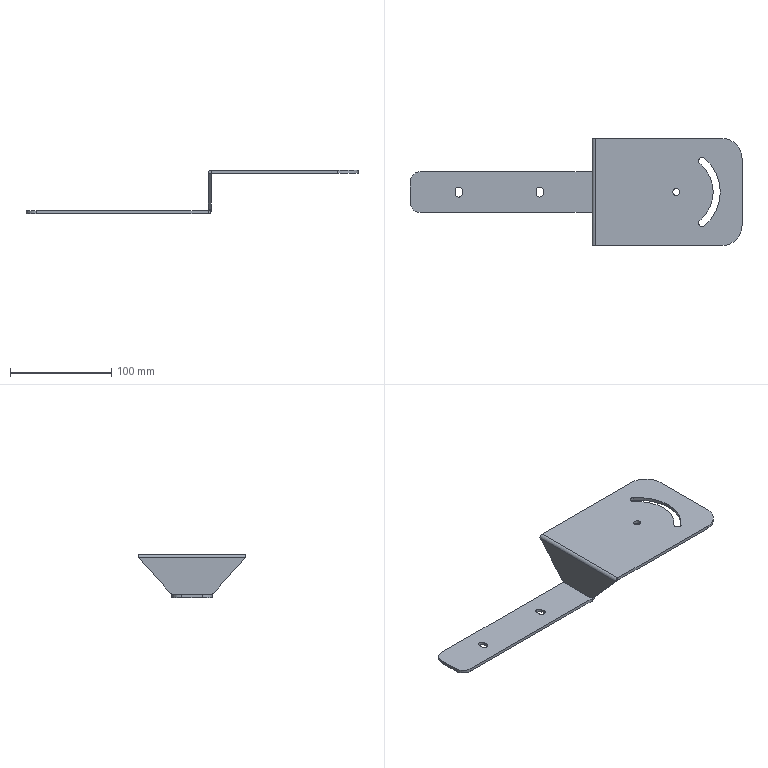Part | STEP file | Tray bracket support plate | 1 solid | 46 faces | box 328 x 106 x 43 mm | volume 74121 mm3 | plane 24 | cylinder 20 | spline 2 | commonest cylinder face diameters 7 x8 0.2 x2 6.2 x2 20 x2 40 x2 73 x2